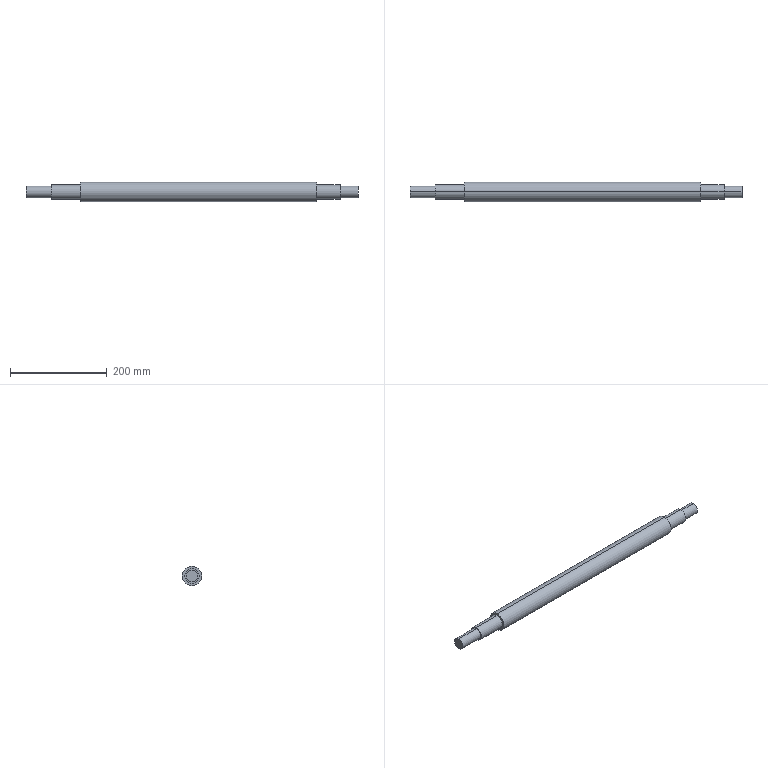Part | SolidWorks | features Revolution 1 | 1 solid | 16 faces | box 685 x 40 x 40 mm | volume 729842 mm3 | cylinder 10 | plane 6 | commonest cylinder face diameters 24 x4 30 x4 40 x2
STEP:
#1=CARTESIAN_POINT('',(590.29,0.,12.));
#2=VERTEX_POINT('',#1);
#3=CARTESIAN_POINT('',(590.29,0.,-12.));
#4=VERTEX_POINT('',#3);
#5=CARTESIAN_POINT('',(590.29,0.,0.));
#6=DIRECTION('',(-1.,0.,0.));
#7=DIRECTION('',(0.,0.,1.));
#8=AXIS2_PLACEMENT_3D('',#5,#6,#7);
#9=CIRCLE('',#8,12.);
#10=EDGE_CURVE('',#2,#4,#9,.T.);
#11=ORIENTED_EDGE('',*,*,#10,.T.);
#12=CARTESIAN_POINT('',(553.29,0.,-12.));
#13=VERTEX_POINT('',#12);
#14=CARTESIAN_POINT('',(-124.903,0.,-12.));
#15=DIRECTION('',(-1.,0.,0.));
#16=VECTOR('',#15,1000.);
#17=LINE('',#14,#16);
#18=EDGE_CURVE('',#4,#13,#17,.T.);
#19=ORIENTED_EDGE('',*,*,#18,.T.);
#20=CARTESIAN_POINT('',(553.29,0.,12.));
#21=VERTEX_POINT('',#20);
#22=CARTESIAN_POINT('',(553.29,0.,0.));
#23=DIRECTION('',(-1.,0.,0.));
#24=DIRECTION('',(0.,0.,1.));
#25=AXIS2_PLACEMENT_3D('',#22,#23,#24);
#26=CIRCLE('',#25,12.);
#27=EDGE_CURVE('',#21,#13,#26,.T.);
#28=ORIENTED_EDGE('',*,*,#27,.F.);
#29=CARTESIAN_POINT('',(-124.903,0.,12.));
#30=DIRECTION('',(-1.,0.,0.));
#31=VECTOR('',#30,1000.);
#32=LINE('',#29,#31);
#33=EDGE_CURVE('',#2,#21,#32,.T.);
#34=ORIENTED_EDGE('',*,*,#33,.F.);
#35=EDGE_LOOP('',(#11,#19,#28,#34));
#36=FACE_OUTER_BOUND('',#35,.T.);
#37=CARTESIAN_POINT('',(-124.903,0.,0.));
#38=DIRECTION('',(-1.,0.,0.));
#39=DIRECTION('',(0.,0.,1.));
#40=AXIS2_PLACEMENT_3D('',#37,#38,#39);
#41=CYLINDRICAL_SURFACE('',#40,12.);
#42=ADVANCED_FACE('',(#36),#41,.T.);
#43=CARTESIAN_POINT('',(553.29,0.,15.));
#44=VERTEX_POINT('',#43);
#45=CARTESIAN_POINT('',(553.29,0.,-15.));
#46=VERTEX_POINT('',#45);
#47=CARTESIAN_POINT('',(553.29,0.,0.));
#48=DIRECTION('',(-1.,0.,0.));
#49=DIRECTION('',(0.,0.,1.));
#50=AXIS2_PLACEMENT_3D('',#47,#48,#49);
#51=CIRCLE('',#50,15.);
#52=EDGE_CURVE('',#44,#46,#51,.T.);
#53=ORIENTED_EDGE('',*,*,#52,.T.);
#54=CARTESIAN_POINT('',(505.29,0.,-15.));
#55=VERTEX_POINT('',#54);
#56=CARTESIAN_POINT('',(-124.903,0.,-15.));
#57=DIRECTION('',(-1.,0.,0.));
#58=VECTOR('',#57,1000.);
#59=LINE('',#56,#58);
#60=EDGE_CURVE('',#46,#55,#59,.T.);
#61=ORIENTED_EDGE('',*,*,#60,.T.);
#62=CARTESIAN_POINT('',(505.29,0.,15.));
#63=VERTEX_POINT('',#62);
#64=CARTESIAN_POINT('',(505.29,0.,0.));
#65=DIRECTION('',(-1.,0.,0.));
#66=DIRECTION('',(0.,0.,1.));
#67=AXIS2_PLACEMENT_3D('',#64,#65,#66);
#68=CIRCLE('',#67,15.);
#69=EDGE_CURVE('',#63,#55,#68,.T.);
#70=ORIENTED_EDGE('',*,*,#69,.F.);
#71=CARTESIAN_POINT('',(-124.903,0.,15.));
#72=DIRECTION('',(-1.,0.,0.));
#73=VECTOR('',#72,1000.);
#74=LINE('',#71,#73);
#75=EDGE_CURVE('',#44,#63,#74,.T.);
#76=ORIENTED_EDGE('',*,*,#75,.F.);
#77=EDGE_LOOP('',(#53,#61,#70,#76));
#78=FACE_OUTER_BOUND('',#77,.T.);
#79=CARTESIAN_POINT('',(-124.903,0.,0.));
#80=DIRECTION('',(-1.,0.,0.));
#81=DIRECTION('',(0.,0.,1.));
#82=AXIS2_PLACEMENT_3D('',#79,#80,#81);
#83=CYLINDRICAL_SURFACE('',#82,15.);
#84=ADVANCED_FACE('',(#78),#83,.T.);
#85=CARTESIAN_POINT('',(505.29,0.,20.));
#86=VERTEX_POINT('',#85);
#87=CARTESIAN_POINT('',(505.29,0.,-20.));
#88=VERTEX_POINT('',#87);
#89=CARTESIAN_POINT('',(505.29,0.,0.));
#90=DIRECTION('',(-1.,0.,0.));
#91=DIRECTION('',(0.,0.,1.));
#92=AXIS2_PLACEMENT_3D('',#89,#90,#91);
#93=CIRCLE('',#92,20.);
#94=EDGE_CURVE('',#86,#88,#93,.T.);
#95=ORIENTED_EDGE('',*,*,#94,.T.);
#96=CARTESIAN_POINT('',(17.29,0.,-20.));
#97=VERTEX_POINT('',#96);
#98=CARTESIAN_POINT('',(-124.903,0.,-20.));
#99=DIRECTION('',(-1.,0.,0.));
#100=VECTOR('',#99,1000.);
#101=LINE('',#98,#100);
#102=EDGE_CURVE('',#88,#97,#101,.T.);
#103=ORIENTED_EDGE('',*,*,#102,.T.);
#104=CARTESIAN_POINT('',(17.29,0.,20.));
#105=VERTEX_POINT('',#104);
#106=CARTESIAN_POINT('',(17.29,0.,0.));
#107=DIRECTION('',(-1.,0.,0.));
#108=DIRECTION('',(0.,0.,1.));
#109=AXIS2_PLACEMENT_3D('',#106,#107,#108);
#110=CIRCLE('',#109,20.);
#111=EDGE_CURVE('',#105,#97,#110,.T.);
#112=ORIENTED_EDGE('',*,*,#111,.F.);
#113=CARTESIAN_POINT('',(-124.903,0.,20.));
#114=DIRECTION('',(-1.,0.,0.));
#115=VECTOR('',#114,1000.);
#116=LINE('',#113,#115);
#117=EDGE_CURVE('',#86,#105,#116,.T.);
#118=ORIENTED_EDGE('',*,*,#117,.F.);
#119=EDGE_LOOP('',(#95,#103,#112,#118));
#120=FACE_OUTER_BOUND('',#119,.T.);
#121=CARTESIAN_POINT('',(-124.903,0.,0.));
#122=DIRECTION('',(-1.,0.,0.));
#123=DIRECTION('',(0.,0.,1.));
#124=AXIS2_PLACEMENT_3D('',#121,#122,#123);
#125=CYLINDRICAL_SURFACE('',#124,20.);
#126=ADVANCED_FACE('',(#120),#125,.T.);
#127=CARTESIAN_POINT('',(17.29,0.,15.));
#128=VERTEX_POINT('',#127);
#129=CARTESIAN_POINT('',(17.29,0.,-15.));
#130=VERTEX_POINT('',#129);
#131=CARTESIAN_POINT('',(17.29,0.,0.));
#132=DIRECTION('',(-1.,0.,0.));
#133=DIRECTION('',(0.,0.,1.));
#134=AXIS2_PLACEMENT_3D('',#131,#132,#133);
#135=CIRCLE('',#134,15.);
#136=EDGE_CURVE('',#128,#130,#135,.T.);
#137=ORIENTED_EDGE('',*,*,#136,.T.);
#138=CARTESIAN_POINT('',(-42.71,0.,-15.));
#139=VERTEX_POINT('',#138);
#140=CARTESIAN_POINT('',(-124.903,0.,-15.));
#141=DIRECTION('',(-1.,0.,0.));
#142=VECTOR('',#141,1000.);
#143=LINE('',#140,#142);
#144=EDGE_CURVE('',#130,#139,#143,.T.);
#145=ORIENTED_EDGE('',*,*,#144,.T.);
#146=CARTESIAN_POINT('',(-42.71,0.,15.));
#147=VERTEX_POINT('',#146);
#148=CARTESIAN_POINT('',(-42.71,0.,0.));
#149=DIRECTION('',(-1.,0.,0.));
#150=DIRECTION('',(0.,0.,1.));
#151=AXIS2_PLACEMENT_3D('',#148,#149,#150);
#152=CIRCLE('',#151,15.);
#153=EDGE_CURVE('',#147,#139,#152,.T.);
#154=ORIENTED_EDGE('',*,*,#153,.F.);
#155=CARTESIAN_POINT('',(-124.903,0.,15.));
#156=DIRECTION('',(-1.,0.,0.));
#157=VECTOR('',#156,1000.);
#158=LINE('',#155,#157);
#159=EDGE_CURVE('',#128,#147,#158,.T.);
#160=ORIENTED_EDGE('',*,*,#159,.F.);
#161=EDGE_LOOP('',(#137,#145,#154,#160));
#162=FACE_OUTER_BOUND('',#161,.T.);
#163=CARTESIAN_POINT('',(-124.903,0.,0.));
#164=DIRECTION('',(-1.,0.,0.));
#165=DIRECTION('',(0.,0.,1.));
#166=AXIS2_PLACEMENT_3D('',#163,#164,#165);
#167=CYLINDRICAL_SURFACE('',#166,15.);
#168=ADVANCED_FACE('',(#162),#167,.T.);
#169=CARTESIAN_POINT('',(-42.71,0.,12.));
#170=VERTEX_POINT('',#169);
#171=CARTESIAN_POINT('',(-42.71,0.,-12.));
#172=VERTEX_POINT('',#171);
#173=CARTESIAN_POINT('',(-42.71,0.,0.));
#174=DIRECTION('',(-1.,0.,0.));
#175=DIRECTION('',(0.,0.,1.));
#176=AXIS2_PLACEMENT_3D('',#173,#174,#175);
#177=CIRCLE('',#176,12.);
#178=EDGE_CURVE('',#170,#172,#177,.T.);
#179=ORIENTED_EDGE('',*,*,#178,.T.);
#180=CARTESIAN_POINT('',(-94.71,0.,-12.));
#181=VERTEX_POINT('',#180);
#182=CARTESIAN_POINT('',(-124.903,0.,-12.));
#183=DIRECTION('',(-1.,0.,0.));
#184=VECTOR('',#183,1000.);
#185=LINE('',#182,#184);
#186=EDGE_CURVE('',#172,#181,#185,.T.);
#187=ORIENTED_EDGE('',*,*,#186,.T.);
#188=CARTESIAN_POINT('',(-94.71,0.,12.));
#189=VERTEX_POINT('',#188);
#190=CARTESIAN_POINT('',(-94.71,0.,0.));
#191=DIRECTION('',(-1.,0.,0.));
#192=DIRECTION('',(0.,0.,1.));
#193=AXIS2_PLACEMENT_3D('',#190,#191,#192);
#194=CIRCLE('',#193,12.);
#195=EDGE_CURVE('',#189,#181,#194,.T.);
#196=ORIENTED_EDGE('',*,*,#195,.F.);
#197=CARTESIAN_POINT('',(-124.903,0.,12.));
#198=DIRECTION('',(-1.,0.,0.));
#199=VECTOR('',#198,1000.);
#200=LINE('',#197,#199);
#201=EDGE_CURVE('',#170,#189,#200,.T.);
#202=ORIENTED_EDGE('',*,*,#201,.F.);
#203=EDGE_LOOP('',(#179,#187,#196,#202));
#204=FACE_OUTER_BOUND('',#203,.T.);
#205=CARTESIAN_POINT('',(-124.903,0.,0.));
#206=DIRECTION('',(-1.,0.,0.));
#207=DIRECTION('',(0.,0.,1.));
#208=AXIS2_PLACEMENT_3D('',#205,#206,#207);
#209=CYLINDRICAL_SURFACE('',#208,12.);
#210=ADVANCED_FACE('',(#204),#209,.T.);
#211=ORIENTED_EDGE('',*,*,#195,.T.);
#212=CARTESIAN_POINT('',(-94.71,0.,0.));
#213=DIRECTION('',(-1.,0.,0.));
#214=DIRECTION('',(0.,0.,1.));
#215=AXIS2_PLACEMENT_3D('',#212,#213,#214);
#216=CIRCLE('',#215,12.);
#217=EDGE_CURVE('',#181,#189,#216,.T.);
#218=ORIENTED_EDGE('',*,*,#217,.T.);
#219=EDGE_LOOP('',(#211,#218));
#220=FACE_OUTER_BOUND('',#219,.T.);
#221=CARTESIAN_POINT('',(-94.71,0.,0.));
#222=DIRECTION('',(1.,0.,0.));
#223=DIRECTION('',(0.,0.,-1.));
#224=AXIS2_PLACEMENT_3D('',#221,#222,#223);
#225=PLANE('',#224);
#226=ADVANCED_FACE('',(#220),#225,.F.);
#227=ORIENTED_EDGE('',*,*,#186,.F.);
#228=CARTESIAN_POINT('',(-42.71,0.,0.));
#229=DIRECTION('',(-1.,0.,0.));
#230=DIRECTION('',(0.,0.,1.));
#231=AXIS2_PLACEMENT_3D('',#228,#229,#230);
#232=CIRCLE('',#231,12.);
#233=EDGE_CURVE('',#172,#170,#232,.T.);
#234=ORIENTED_EDGE('',*,*,#233,.T.);
#235=ORIENTED_EDGE('',*,*,#201,.T.);
#236=ORIENTED_EDGE('',*,*,#217,.F.);
#237=EDGE_LOOP('',(#227,#234,#235,#236));
#238=FACE_OUTER_BOUND('',#237,.T.);
#239=CARTESIAN_POINT('',(-124.903,0.,0.));
#240=DIRECTION('',(-1.,0.,0.));
#241=DIRECTION('',(0.,0.,1.));
#242=AXIS2_PLACEMENT_3D('',#239,#240,#241);
#243=CYLINDRICAL_SURFACE('',#242,12.);
#244=ADVANCED_FACE('',(#238),#243,.T.);
#245=ORIENTED_EDGE('',*,*,#178,.F.);
#246=ORIENTED_EDGE('',*,*,#233,.F.);
#247=EDGE_LOOP('',(#245,#246));
#248=FACE_BOUND('',#247,.T.);
#249=ORIENTED_EDGE('',*,*,#153,.T.);
#250=CARTESIAN_POINT('',(-42.71,0.,0.));
#251=DIRECTION('',(-1.,0.,0.));
#252=DIRECTION('',(0.,0.,1.));
#253=AXIS2_PLACEMENT_3D('',#250,#251,#252);
#254=CIRCLE('',#253,15.);
#255=EDGE_CURVE('',#139,#147,#254,.T.);
#256=ORIENTED_EDGE('',*,*,#255,.T.);
#257=EDGE_LOOP('',(#249,#256));
#258=FACE_OUTER_BOUND('',#257,.T.);
#259=CARTESIAN_POINT('',(-42.71,12.,0.));
#260=DIRECTION('',(1.,0.,0.));
#261=DIRECTION('',(0.,0.,-1.));
#262=AXIS2_PLACEMENT_3D('',#259,#260,#261);
#263=PLANE('',#262);
#264=ADVANCED_FACE('',(#248,#258),#263,.F.);
#265=ORIENTED_EDGE('',*,*,#144,.F.);
#266=CARTESIAN_POINT('',(17.29,0.,0.));
#267=DIRECTION('',(-1.,0.,0.));
#268=DIRECTION('',(0.,0.,1.));
#269=AXIS2_PLACEMENT_3D('',#266,#267,#268);
#270=CIRCLE('',#269,15.);
#271=EDGE_CURVE('',#130,#128,#270,.T.);
#272=ORIENTED_EDGE('',*,*,#271,.T.);
#273=ORIENTED_EDGE('',*,*,#159,.T.);
#274=ORIENTED_EDGE('',*,*,#255,.F.);
#275=EDGE_LOOP('',(#265,#272,#273,#274));
#276=FACE_OUTER_BOUND('',#275,.T.);
#277=CARTESIAN_POINT('',(-124.903,0.,0.));
#278=DIRECTION('',(-1.,0.,0.));
#279=DIRECTION('',(0.,0.,1.));
#280=AXIS2_PLACEMENT_3D('',#277,#278,#279);
#281=CYLINDRICAL_SURFACE('',#280,15.);
#282=ADVANCED_FACE('',(#276),#281,.T.);
#283=ORIENTED_EDGE('',*,*,#136,.F.);
#284=ORIENTED_EDGE('',*,*,#271,.F.);
#285=EDGE_LOOP('',(#283,#284));
#286=FACE_BOUND('',#285,.T.);
#287=ORIENTED_EDGE('',*,*,#111,.T.);
#288=CARTESIAN_POINT('',(17.29,0.,0.));
#289=DIRECTION('',(-1.,0.,0.));
#290=DIRECTION('',(0.,0.,1.));
#291=AXIS2_PLACEMENT_3D('',#288,#289,#290);
#292=CIRCLE('',#291,20.);
#293=EDGE_CURVE('',#97,#105,#292,.T.);
#294=ORIENTED_EDGE('',*,*,#293,.T.);
#295=EDGE_LOOP('',(#287,#294));
#296=FACE_OUTER_BOUND('',#295,.T.);
#297=CARTESIAN_POINT('',(17.29,15.,0.));
#298=DIRECTION('',(1.,0.,0.));
#299=DIRECTION('',(0.,0.,-1.));
#300=AXIS2_PLACEMENT_3D('',#297,#298,#299);
#301=PLANE('',#300);
#302=ADVANCED_FACE('',(#286,#296),#301,.F.);
#303=ORIENTED_EDGE('',*,*,#102,.F.);
#304=CARTESIAN_POINT('',(505.29,0.,0.));
#305=DIRECTION('',(-1.,0.,0.));
#306=DIRECTION('',(0.,0.,1.));
#307=AXIS2_PLACEMENT_3D('',#304,#305,#306);
#308=CIRCLE('',#307,20.);
#309=EDGE_CURVE('',#88,#86,#308,.T.);
#310=ORIENTED_EDGE('',*,*,#309,.T.);
#311=ORIENTED_EDGE('',*,*,#117,.T.);
#312=ORIENTED_EDGE('',*,*,#293,.F.);
#313=EDGE_LOOP('',(#303,#310,#311,#312));
#314=FACE_OUTER_BOUND('',#313,.T.);
#315=CARTESIAN_POINT('',(-124.903,0.,0.));
#316=DIRECTION('',(-1.,0.,0.));
#317=DIRECTION('',(0.,0.,1.));
#318=AXIS2_PLACEMENT_3D('',#315,#316,#317);
#319=CYLINDRICAL_SURFACE('',#318,20.);
#320=ADVANCED_FACE('',(#314),#319,.T.);
#321=ORIENTED_EDGE('',*,*,#94,.F.);
#322=ORIENTED_EDGE('',*,*,#309,.F.);
#323=EDGE_LOOP('',(#321,#322));
#324=FACE_OUTER_BOUND('',#323,.T.);
#325=ORIENTED_EDGE('',*,*,#69,.T.);
#326=CARTESIAN_POINT('',(505.29,0.,0.));
#327=DIRECTION('',(-1.,0.,0.));
#328=DIRECTION('',(0.,0.,1.));
#329=AXIS2_PLACEMENT_3D('',#326,#327,#328);
#330=CIRCLE('',#329,15.);
#331=EDGE_CURVE('',#55,#63,#330,.T.);
#332=ORIENTED_EDGE('',*,*,#331,.T.);
#333=EDGE_LOOP('',(#325,#332));
#334=FACE_BOUND('',#333,.T.);
#335=CARTESIAN_POINT('',(505.29,20.,0.));
#336=DIRECTION('',(-1.,0.,0.));
#337=DIRECTION('',(0.,0.,1.));
#338=AXIS2_PLACEMENT_3D('',#335,#336,#337);
#339=PLANE('',#338);
#340=ADVANCED_FACE('',(#324,#334),#339,.F.);
#341=ORIENTED_EDGE('',*,*,#60,.F.);
#342=CARTESIAN_POINT('',(553.29,0.,0.));
#343=DIRECTION('',(-1.,0.,0.));
#344=DIRECTION('',(0.,0.,1.));
#345=AXIS2_PLACEMENT_3D('',#342,#343,#344);
#346=CIRCLE('',#345,15.);
#347=EDGE_CURVE('',#46,#44,#346,.T.);
#348=ORIENTED_EDGE('',*,*,#347,.T.);
#349=ORIENTED_EDGE('',*,*,#75,.T.);
#350=ORIENTED_EDGE('',*,*,#331,.F.);
#351=EDGE_LOOP('',(#341,#348,#349,#350));
#352=FACE_OUTER_BOUND('',#351,.T.);
#353=CARTESIAN_POINT('',(-124.903,0.,0.));
#354=DIRECTION('',(-1.,0.,0.));
#355=DIRECTION('',(0.,0.,1.));
#356=AXIS2_PLACEMENT_3D('',#353,#354,#355);
#357=CYLINDRICAL_SURFACE('',#356,15.);
#358=ADVANCED_FACE('',(#352),#357,.T.);
#359=ORIENTED_EDGE('',*,*,#52,.F.);
#360=ORIENTED_EDGE('',*,*,#347,.F.);
#361=EDGE_LOOP('',(#359,#360));
#362=FACE_OUTER_BOUND('',#361,.T.);
#363=ORIENTED_EDGE('',*,*,#27,.T.);
#364=CARTESIAN_POINT('',(553.29,0.,0.));
#365=DIRECTION('',(-1.,0.,0.));
#366=DIRECTION('',(0.,0.,1.));
#367=AXIS2_PLACEMENT_3D('',#364,#365,#366);
#368=CIRCLE('',#367,12.);
#369=EDGE_CURVE('',#13,#21,#368,.T.);
#370=ORIENTED_EDGE('',*,*,#369,.T.);
#371=EDGE_LOOP('',(#363,#370));
#372=FACE_BOUND('',#371,.T.);
#373=CARTESIAN_POINT('',(553.29,15.,0.));
#374=DIRECTION('',(-1.,0.,0.));
#375=DIRECTION('',(0.,0.,1.));
#376=AXIS2_PLACEMENT_3D('',#373,#374,#375);
#377=PLANE('',#376);
#378=ADVANCED_FACE('',(#362,#372),#377,.F.);
#379=ORIENTED_EDGE('',*,*,#18,.F.);
#380=CARTESIAN_POINT('',(590.29,0.,0.));
#381=DIRECTION('',(-1.,0.,0.));
#382=DIRECTION('',(0.,0.,1.));
#383=AXIS2_PLACEMENT_3D('',#380,#381,#382);
#384=CIRCLE('',#383,12.);
#385=EDGE_CURVE('',#4,#2,#384,.T.);
#386=ORIENTED_EDGE('',*,*,#385,.T.);
#387=ORIENTED_EDGE('',*,*,#33,.T.);
#388=ORIENTED_EDGE('',*,*,#369,.F.);
#389=EDGE_LOOP('',(#379,#386,#387,#388));
#390=FACE_OUTER_BOUND('',#389,.T.);
#391=CARTESIAN_POINT('',(-124.903,0.,0.));
#392=DIRECTION('',(-1.,0.,0.));
#393=DIRECTION('',(0.,0.,1.));
#394=AXIS2_PLACEMENT_3D('',#391,#392,#393);
#395=CYLINDRICAL_SURFACE('',#394,12.);
#396=ADVANCED_FACE('',(#390),#395,.T.);
#397=ORIENTED_EDGE('',*,*,#10,.F.);
#398=ORIENTED_EDGE('',*,*,#385,.F.);
#399=EDGE_LOOP('',(#397,#398));
#400=FACE_OUTER_BOUND('',#399,.T.);
#401=CARTESIAN_POINT('',(590.29,12.,0.));
#402=DIRECTION('',(-1.,0.,0.));
#403=DIRECTION('',(0.,0.,1.));
#404=AXIS2_PLACEMENT_3D('',#401,#402,#403);
#405=PLANE('',#404);
#406=ADVANCED_FACE('',(#400),#405,.F.);
#407=CLOSED_SHELL('',(#42,#84,#126,#168,#210,#226,#244,#264,#282,#302,#320,#340,#358,#378,#396,#406));
#408=MANIFOLD_SOLID_BREP('',#407);
#409=CARTESIAN_POINT('',(0.,0.,0.));
#410=DIRECTION('',(0.,0.,1.));
#411=DIRECTION('',(1.,0.,0.));
#412=AXIS2_PLACEMENT_3D('',#409,#410,#411);
#413=(LENGTH_UNIT()NAMED_UNIT(*)SI_UNIT(.MILLI.,.METRE.));
#414=UNCERTAINTY_MEASURE_WITH_UNIT(LENGTH_MEASURE(0.00001),#413,'','');
#415=(NAMED_UNIT(*)PLANE_ANGLE_UNIT()SI_UNIT($,.RADIAN.));
#416=(NAMED_UNIT(*)SI_UNIT($,.STERADIAN.)SOLID_ANGLE_UNIT());
#417=(GEOMETRIC_REPRESENTATION_CONTEXT(3)GLOBAL_UNCERTAINTY_ASSIGNED_CONTEXT((#414))GLOBAL_UNIT_ASSIGNED_CONTEXT((#413,#415,#416))REPRESENTATION_CONTEXT('',''));
#418=ADVANCED_BREP_SHAPE_REPRESENTATION('',(#408,#412),#417);